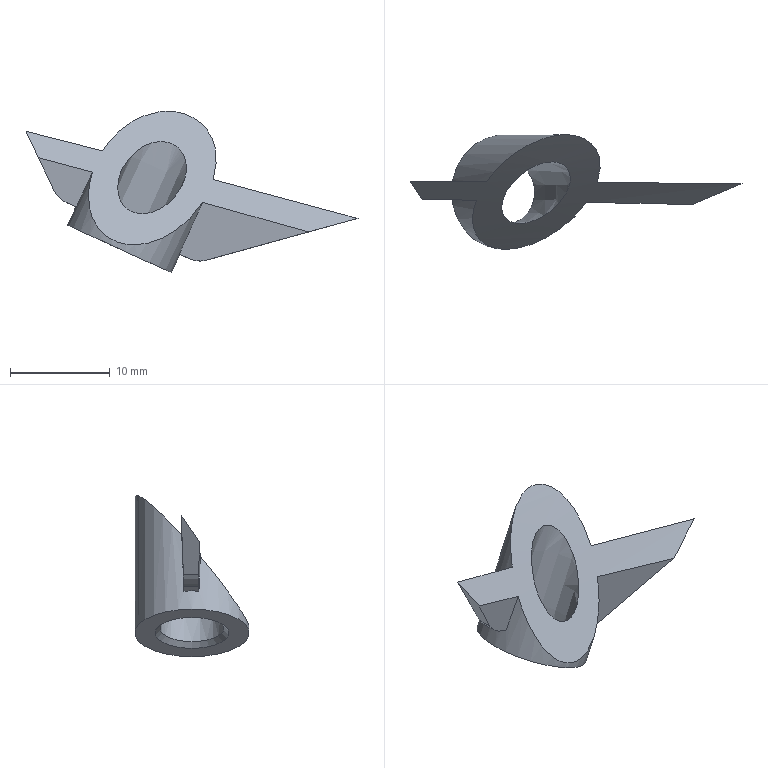Part | STEP file | solid 274 | 1 solid | 15 faces | box 33.29 x 11.457 x 16.18 mm | volume 703.754 mm3 | plane 9 | cylinder 3 | cone 2 | spline 1 | commonest cylinder face diameters 5.025 x2 11.457 x1